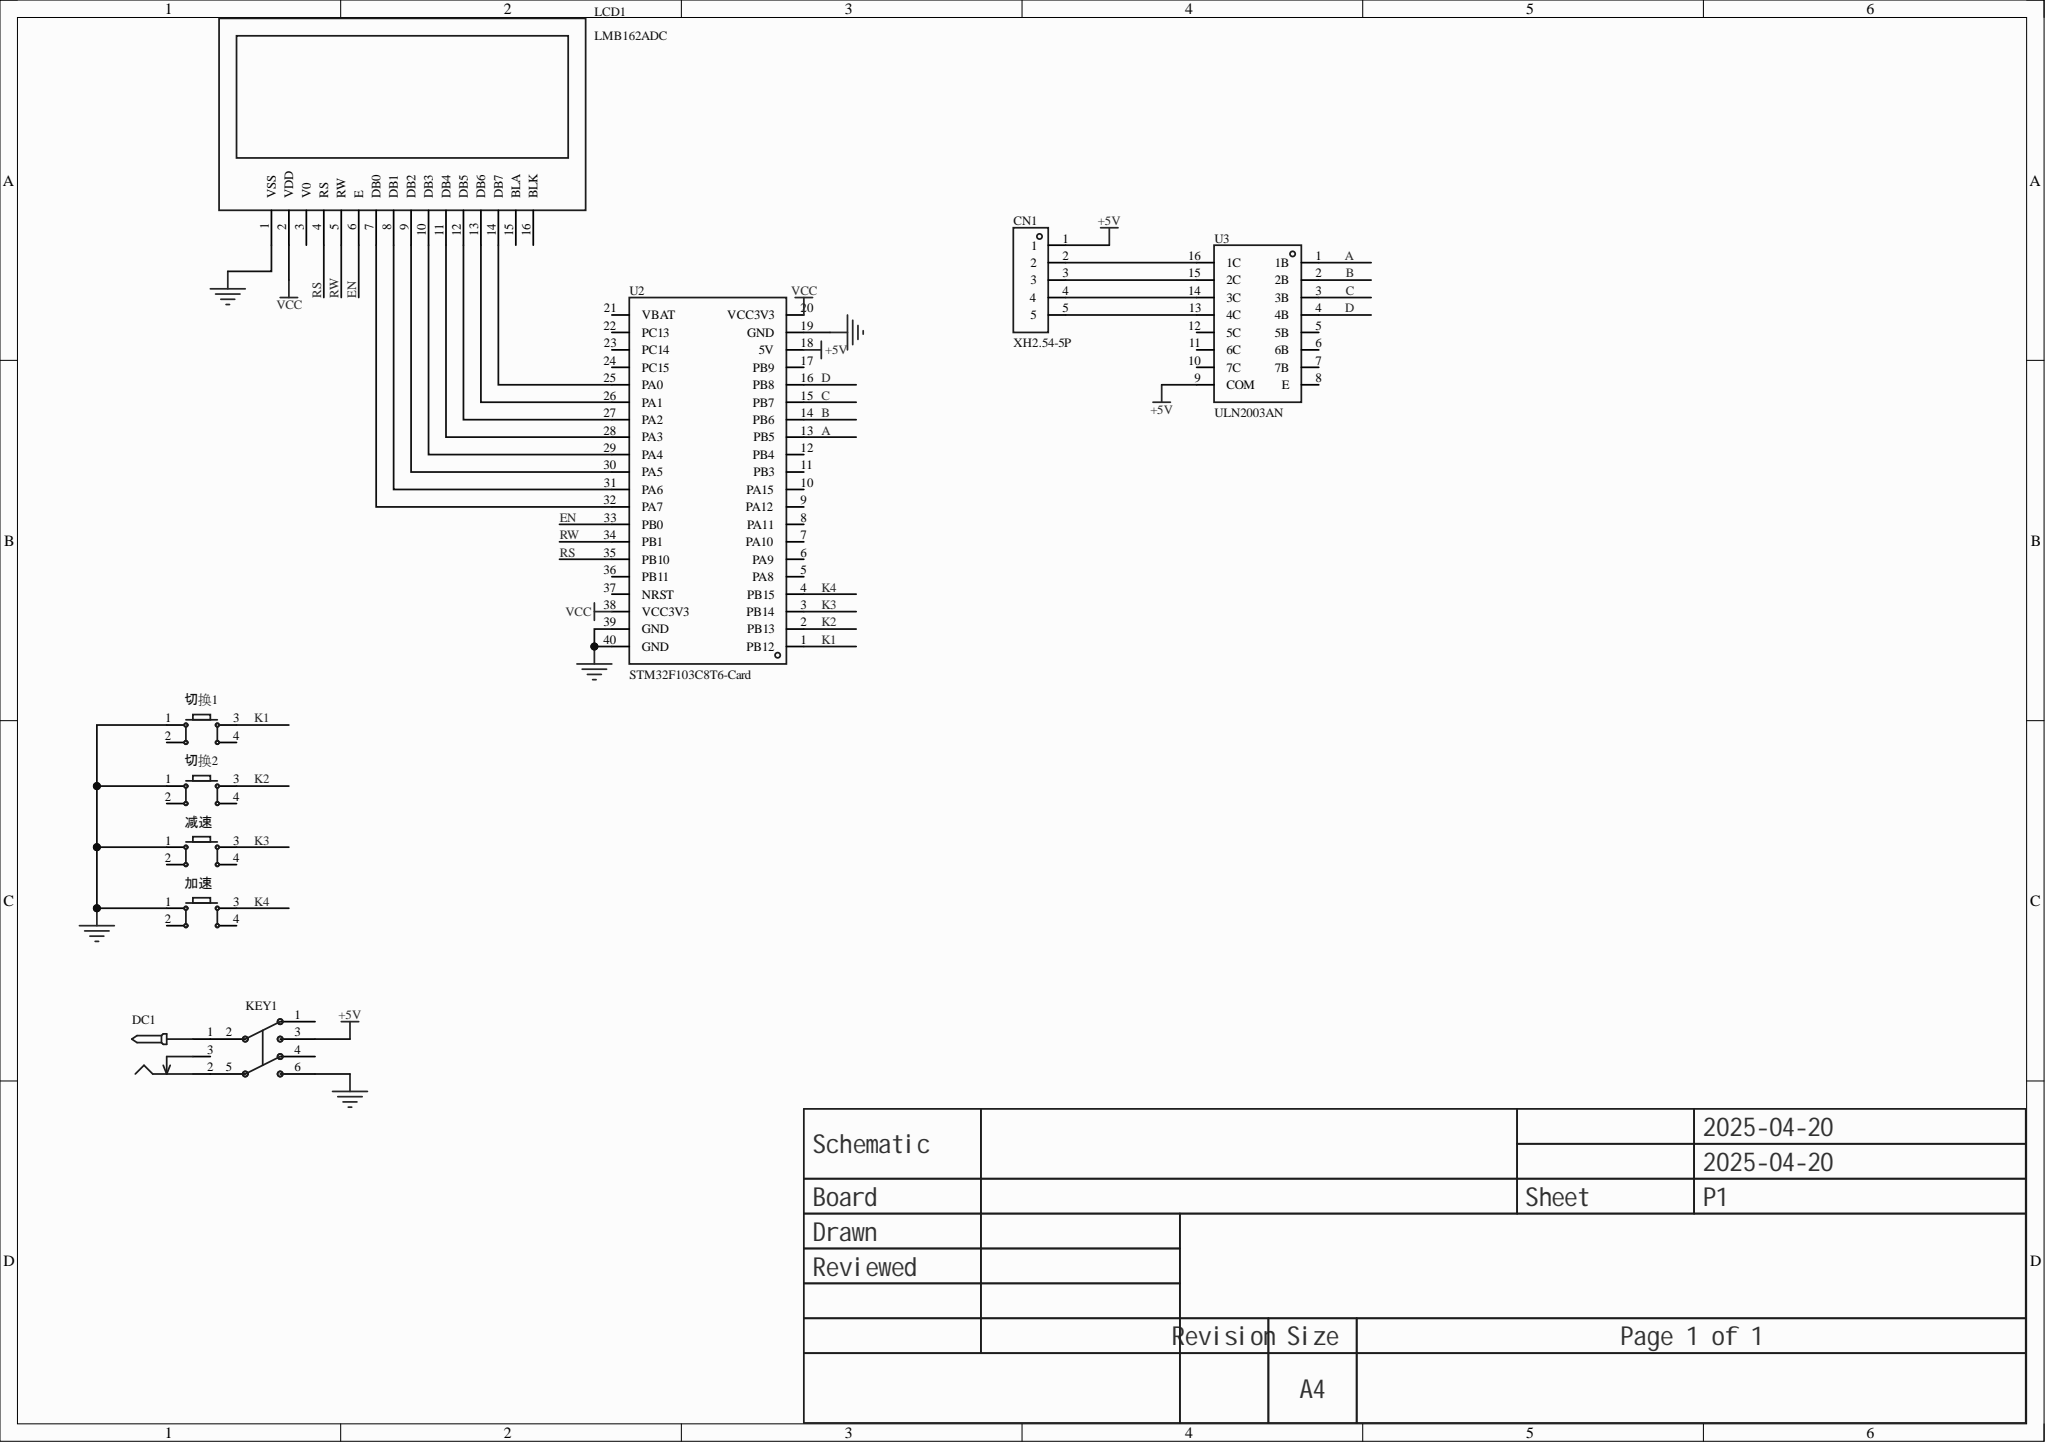Circuit board | Altium Designer | 10 parts | 28 nets
Bill of materials:
Comment,Description,Designator,Footprint,LibRef,Quantity
"XH2.54-5P","","CN1","CONN-TH_5P-P2.54_C9900008095","XH2.54-5P","1"
"","","DC1","DC-005_2.5","DC-005_2.5","1"
"Non-latching switch 8.5×8.5, silent","6 pins, 8.5×8.5","KEY1","SW-TH_6P-L8.5-W8.5-P2.54","无自锁开关 8.5×8.5 无声","1"
"LMB162ADC","16x2 character LCD module","LCD1","LCD1602","LMB162ADC","1"
"STM32F103C8T6-Card","","U2","CONN-TH_L53.3-W22.9_STM32F103C8T6-CARD","STM32F103C8T6-Card","1"
"ULN2003AN","通道数:七路;集射击穿电压(Vceo):50V;","U3","DIP-16_L19.8-W6.5-P2.54-LS7.6-BL","ULN2003AN","1"
"","","减速, 切换1, 切换2, 加速","SW-TH_4P-L6.0-W6.0-P4.50-LS6.5","Key_TH_6x6x6","4"
Netlist (Protel format):
[
CN1
CONN-TH_5P-P2.54_C9900008095
XH2.54-5P



]
[
DC1
DC-005_2.5




]
[
KEY1
SW-TH_6P-L8.5-W8.5-P2.54
Non-latching switch 8.5×8.5, silent



]
[
LCD1
LCD1602
LMB162ADC



]
[
U2
CONN-TH_L53.3-W22.9_STM32F103C8T6-CARD
STM32F103C8T6-Card



]
[
U3
DIP-16_L19.8-W6.5-P2.54-LS7.6-BL
ULN2003AN



]
[
减速
SW-TH_4P-L6.0-W6.0-P4.50-LS6.5




]
[
切换1
SW-TH_4P-L6.0-W6.0-P4.50-LS6.5




]
[
切换2
SW-TH_4P-L6.0-W6.0-P4.50-LS6.5




]
[
加速
SW-TH_4P-L6.0-W6.0-P4.50-LS6.5




]
(
VCC
LCD1-2
U2-20
U2-38
)
(
RW
LCD1-5
U2-34
)
(
RS
LCD1-4
U2-35
)
(
NetLCD1_14
LCD1-14
U2-25
)
(
NetLCD1_13
LCD1-13
U2-26
)
(
NetLCD1_12
LCD1-12
U2-27
)
(
NetLCD1_11
LCD1-11
U2-28
)
(
NetLCD1_10
LCD1-10
U2-29
)
(
NetLCD1_9
LCD1-9
U2-30
)
(
NetLCD1_8
LCD1-8
U2-31
)
(
NetLCD1_7
LCD1-7
U2-32
)
(
NetDC1_2
DC1-2
KEY1-5
)
(
NetDC1_1
DC1-1
KEY1-2
)
(
NetCN1_5
CN1-5
U3-13
)
(
NetCN1_4
CN1-4
U3-14
)
(
NetCN1_3
CN1-3
U3-15
)
(
NetCN1_2
CN1-2
U3-16
)
(
K4
U2-4
加速-3
)
(
K3
U2-3
减速-3
)
(
K2
U2-2
切换2-3
)
(
K1
U2-1
切换1-3
)
(
GND
KEY1-6
LCD1-1
U2-19
U2-39
U2-40
减速-1
切换1-1
切换2-1
加速-1
)
(
EN
LCD1-6
U2-33
)
(
D
U2-16
U3-4
)
(
C
U2-15
U3-3
)
(
B
U2-14
U3-2
)
(
A
U2-13
U3-1
)
(
+5V
CN1-1
KEY1-3
U2-18
U3-9
)